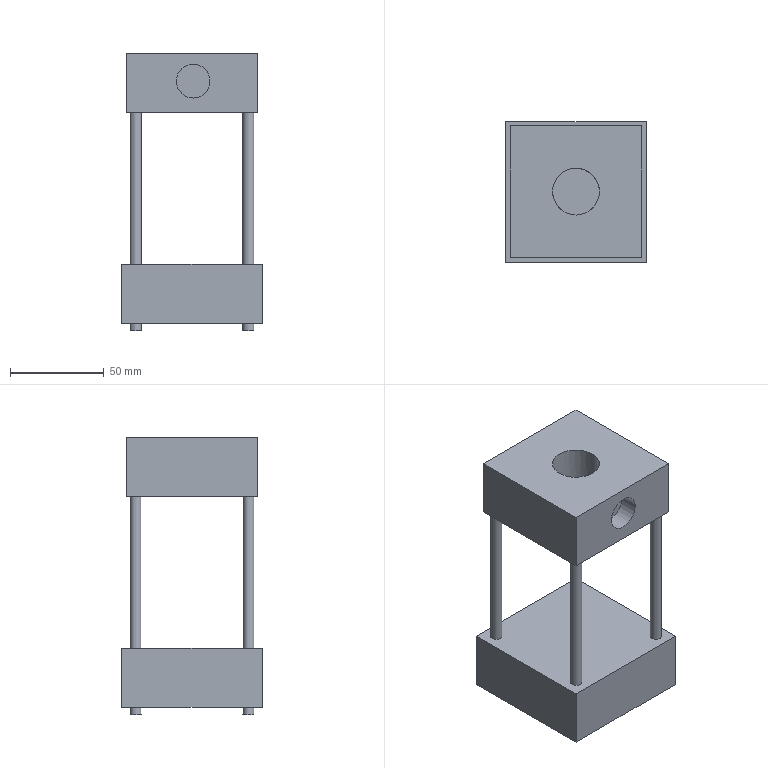Part | NX | features solid 2 | 1 solid | 27 faces | box 75 x 75 x 148 mm | volume 323144 mm3 | plane 17 | cylinder 10 | commonest cylinder face diameters 6 x8 18 x1 25 x1
STEP:
#1=CARTESIAN_POINT('',(33.,-470.,-344.));
#2=VERTEX_POINT('',#1);
#3=CARTESIAN_POINT('',(30.,-470.,-344.));
#4=DIRECTION('',(0.,0.,1.));
#5=DIRECTION('',(1.,0.,0.));
#6=AXIS2_PLACEMENT_3D('',#3,#4,#5);
#7=CIRCLE('',#6,3.);
#8=EDGE_CURVE('',#2,#2,#7,.T.);
#9=ORIENTED_EDGE('',*,*,#8,.T.);
#10=EDGE_LOOP('',(#9));
#11=FACE_BOUND('',#10,.T.);
#12=CARTESIAN_POINT('',(-27.,-410.,-344.));
#13=VERTEX_POINT('',#12);
#14=CARTESIAN_POINT('',(-30.,-410.,-344.));
#15=DIRECTION('',(0.,0.,1.));
#16=DIRECTION('',(1.,0.,0.));
#17=AXIS2_PLACEMENT_3D('',#14,#15,#16);
#18=CIRCLE('',#17,3.);
#19=EDGE_CURVE('',#13,#13,#18,.T.);
#20=ORIENTED_EDGE('',*,*,#19,.T.);
#21=EDGE_LOOP('',(#20));
#22=FACE_BOUND('',#21,.T.);
#23=CARTESIAN_POINT('',(-5.146,-477.5,-344.));
#24=VERTEX_POINT('',#23);
#25=CARTESIAN_POINT('',(-5.146,-465.,-344.));
#26=VERTEX_POINT('',#25);
#27=CARTESIAN_POINT('',(-5.146,-475.,-344.));
#28=DIRECTION('',(0.,1.,0.));
#29=VECTOR('',#28,1000.);
#30=LINE('',#27,#29);
#31=EDGE_CURVE('',#24,#26,#30,.T.);
#32=ORIENTED_EDGE('',*,*,#31,.F.);
#33=CARTESIAN_POINT('',(-37.5,-477.5,-344.));
#34=VERTEX_POINT('',#33);
#35=CARTESIAN_POINT('',(-35.,-477.5,-344.));
#36=DIRECTION('',(-1.,0.,0.));
#37=VECTOR('',#36,1000.);
#38=LINE('',#35,#37);
#39=EDGE_CURVE('',#24,#34,#38,.T.);
#40=ORIENTED_EDGE('',*,*,#39,.T.);
#41=CARTESIAN_POINT('',(-37.5,-402.5,-344.));
#42=VERTEX_POINT('',#41);
#43=CARTESIAN_POINT('',(-37.5,-475.,-344.));
#44=DIRECTION('',(0.,1.,0.));
#45=VECTOR('',#44,1000.);
#46=LINE('',#43,#45);
#47=EDGE_CURVE('',#42,#34,#46,.F.);
#48=ORIENTED_EDGE('',*,*,#47,.F.);
#49=CARTESIAN_POINT('',(37.5,-402.5,-344.));
#50=VERTEX_POINT('',#49);
#51=CARTESIAN_POINT('',(-35.,-402.5,-344.));
#52=DIRECTION('',(1.,0.,0.));
#53=VECTOR('',#52,1000.);
#54=LINE('',#51,#53);
#55=EDGE_CURVE('',#50,#42,#54,.F.);
#56=ORIENTED_EDGE('',*,*,#55,.F.);
#57=CARTESIAN_POINT('',(37.5,-477.5,-344.));
#58=VERTEX_POINT('',#57);
#59=CARTESIAN_POINT('',(37.5,-475.,-344.));
#60=DIRECTION('',(0.,-1.,0.));
#61=VECTOR('',#60,1000.);
#62=LINE('',#59,#61);
#63=EDGE_CURVE('',#58,#50,#62,.F.);
#64=ORIENTED_EDGE('',*,*,#63,.F.);
#65=CARTESIAN_POINT('',(3.1,-477.5,-344.));
#66=VERTEX_POINT('',#65);
#67=CARTESIAN_POINT('',(-35.,-477.5,-344.));
#68=DIRECTION('',(-1.,0.,0.));
#69=VECTOR('',#68,1000.);
#70=LINE('',#67,#69);
#71=EDGE_CURVE('',#58,#66,#70,.T.);
#72=ORIENTED_EDGE('',*,*,#71,.T.);
#73=CARTESIAN_POINT('',(3.1,-465.,-344.));
#74=VERTEX_POINT('',#73);
#75=CARTESIAN_POINT('',(3.1,-475.,-344.));
#76=DIRECTION('',(0.,1.,0.));
#77=VECTOR('',#76,1000.);
#78=LINE('',#75,#77);
#79=EDGE_CURVE('',#66,#74,#78,.T.);
#80=ORIENTED_EDGE('',*,*,#79,.T.);
#81=ORIENTED_EDGE('',*,*,#79,.F.);
#82=CARTESIAN_POINT('',(-35.,-477.5,-344.));
#83=DIRECTION('',(1.,0.,0.));
#84=VECTOR('',#83,1000.);
#85=LINE('',#82,#84);
#86=EDGE_CURVE('',#66,#24,#85,.F.);
#87=ORIENTED_EDGE('',*,*,#86,.T.);
#88=ORIENTED_EDGE('',*,*,#31,.T.);
#89=EDGE_LOOP('',(#32,#40,#48,#56,#64,#72,#80,#81,#87,#88));
#90=FACE_BOUND('',#89,.T.);
#91=CARTESIAN_POINT('',(-27.,-470.,-344.));
#92=VERTEX_POINT('',#91);
#93=CARTESIAN_POINT('',(-30.,-470.,-344.));
#94=DIRECTION('',(0.,0.,1.));
#95=DIRECTION('',(1.,0.,0.));
#96=AXIS2_PLACEMENT_3D('',#93,#94,#95);
#97=CIRCLE('',#96,3.);
#98=EDGE_CURVE('',#92,#92,#97,.T.);
#99=ORIENTED_EDGE('',*,*,#98,.T.);
#100=EDGE_LOOP('',(#99));
#101=FACE_BOUND('',#100,.T.);
#102=CARTESIAN_POINT('',(33.,-410.,-344.));
#103=VERTEX_POINT('',#102);
#104=CARTESIAN_POINT('',(30.,-410.,-344.));
#105=DIRECTION('',(0.,0.,1.));
#106=DIRECTION('',(1.,0.,0.));
#107=AXIS2_PLACEMENT_3D('',#104,#105,#106);
#108=CIRCLE('',#107,3.);
#109=EDGE_CURVE('',#103,#103,#108,.T.);
#110=ORIENTED_EDGE('',*,*,#109,.T.);
#111=EDGE_LOOP('',(#110));
#112=FACE_BOUND('',#111,.T.);
#113=CARTESIAN_POINT('',(-35.,-475.,-344.));
#114=DIRECTION('',(0.,0.,-1.));
#115=DIRECTION('',(1.,0.,0.));
#116=AXIS2_PLACEMENT_3D('',#113,#114,#115);
#117=PLANE('',#116);
#118=ADVANCED_FACE('',(#11,#22,#90,#101,#112),#117,.T.);
#119=CARTESIAN_POINT('',(-27.,-470.,-231.5));
#120=VERTEX_POINT('',#119);
#121=CARTESIAN_POINT('',(-30.,-470.,-231.5));
#122=DIRECTION('',(0.,0.,1.));
#123=DIRECTION('',(1.,0.,0.));
#124=AXIS2_PLACEMENT_3D('',#121,#122,#123);
#125=CIRCLE('',#124,3.);
#126=EDGE_CURVE('',#120,#120,#125,.T.);
#127=ORIENTED_EDGE('',*,*,#126,.F.);
#128=EDGE_LOOP('',(#127));
#129=FACE_BOUND('',#128,.T.);
#130=CARTESIAN_POINT('',(-27.,-470.,-312.5));
#131=VERTEX_POINT('',#130);
#132=CARTESIAN_POINT('',(-30.,-470.,-312.5));
#133=DIRECTION('',(0.,0.,1.));
#134=DIRECTION('',(1.,0.,0.));
#135=AXIS2_PLACEMENT_3D('',#132,#133,#134);
#136=CIRCLE('',#135,3.);
#137=EDGE_CURVE('',#131,#131,#136,.F.);
#138=ORIENTED_EDGE('',*,*,#137,.F.);
#139=EDGE_LOOP('',(#138));
#140=FACE_BOUND('',#139,.T.);
#141=CARTESIAN_POINT('',(-30.,-470.,-486.));
#142=DIRECTION('',(0.,0.,1.));
#143=DIRECTION('',(-1.,0.,0.));
#144=AXIS2_PLACEMENT_3D('',#141,#142,#143);
#145=CYLINDRICAL_SURFACE('',#144,3.);
#146=ADVANCED_FACE('',(#129,#140),#145,.T.);
#147=CARTESIAN_POINT('',(33.,-470.,-231.5));
#148=VERTEX_POINT('',#147);
#149=CARTESIAN_POINT('',(30.,-470.,-231.5));
#150=DIRECTION('',(0.,0.,1.));
#151=DIRECTION('',(1.,0.,0.));
#152=AXIS2_PLACEMENT_3D('',#149,#150,#151);
#153=CIRCLE('',#152,3.);
#154=EDGE_CURVE('',#148,#148,#153,.F.);
#155=ORIENTED_EDGE('',*,*,#154,.T.);
#156=EDGE_LOOP('',(#155));
#157=FACE_BOUND('',#156,.T.);
#158=CARTESIAN_POINT('',(33.,-470.,-312.5));
#159=VERTEX_POINT('',#158);
#160=CARTESIAN_POINT('',(30.,-470.,-312.5));
#161=DIRECTION('',(0.,0.,1.));
#162=DIRECTION('',(1.,0.,0.));
#163=AXIS2_PLACEMENT_3D('',#160,#161,#162);
#164=CIRCLE('',#163,3.);
#165=EDGE_CURVE('',#159,#159,#164,.T.);
#166=ORIENTED_EDGE('',*,*,#165,.T.);
#167=EDGE_LOOP('',(#166));
#168=FACE_BOUND('',#167,.T.);
#169=CARTESIAN_POINT('',(30.,-470.,-486.));
#170=DIRECTION('',(0.,0.,1.));
#171=DIRECTION('',(-1.,0.,0.));
#172=AXIS2_PLACEMENT_3D('',#169,#170,#171);
#173=CYLINDRICAL_SURFACE('',#172,3.);
#174=ADVANCED_FACE('',(#157,#168),#173,.T.);
#175=CARTESIAN_POINT('',(33.,-410.,-231.5));
#176=VERTEX_POINT('',#175);
#177=CARTESIAN_POINT('',(30.,-410.,-231.5));
#178=DIRECTION('',(0.,0.,1.));
#179=DIRECTION('',(1.,0.,0.));
#180=AXIS2_PLACEMENT_3D('',#177,#178,#179);
#181=CIRCLE('',#180,3.);
#182=EDGE_CURVE('',#176,#176,#181,.T.);
#183=ORIENTED_EDGE('',*,*,#182,.F.);
#184=EDGE_LOOP('',(#183));
#185=FACE_BOUND('',#184,.T.);
#186=CARTESIAN_POINT('',(33.,-410.,-312.5));
#187=VERTEX_POINT('',#186);
#188=CARTESIAN_POINT('',(30.,-410.,-312.5));
#189=DIRECTION('',(0.,0.,1.));
#190=DIRECTION('',(1.,0.,0.));
#191=AXIS2_PLACEMENT_3D('',#188,#189,#190);
#192=CIRCLE('',#191,3.);
#193=EDGE_CURVE('',#187,#187,#192,.F.);
#194=ORIENTED_EDGE('',*,*,#193,.F.);
#195=EDGE_LOOP('',(#194));
#196=FACE_BOUND('',#195,.T.);
#197=CARTESIAN_POINT('',(30.,-410.,-486.));
#198=DIRECTION('',(0.,0.,1.));
#199=DIRECTION('',(-1.,0.,0.));
#200=AXIS2_PLACEMENT_3D('',#197,#198,#199);
#201=CYLINDRICAL_SURFACE('',#200,3.);
#202=ADVANCED_FACE('',(#185,#196),#201,.T.);
#203=CARTESIAN_POINT('',(-27.,-410.,-231.5));
#204=VERTEX_POINT('',#203);
#205=CARTESIAN_POINT('',(-30.,-410.,-231.5));
#206=DIRECTION('',(0.,0.,1.));
#207=DIRECTION('',(1.,0.,0.));
#208=AXIS2_PLACEMENT_3D('',#205,#206,#207);
#209=CIRCLE('',#208,3.);
#210=EDGE_CURVE('',#204,#204,#209,.F.);
#211=ORIENTED_EDGE('',*,*,#210,.T.);
#212=EDGE_LOOP('',(#211));
#213=FACE_BOUND('',#212,.T.);
#214=CARTESIAN_POINT('',(-27.,-410.,-312.5));
#215=VERTEX_POINT('',#214);
#216=CARTESIAN_POINT('',(-30.,-410.,-312.5));
#217=DIRECTION('',(0.,0.,1.));
#218=DIRECTION('',(1.,0.,0.));
#219=AXIS2_PLACEMENT_3D('',#216,#217,#218);
#220=CIRCLE('',#219,3.);
#221=EDGE_CURVE('',#215,#215,#220,.T.);
#222=ORIENTED_EDGE('',*,*,#221,.T.);
#223=EDGE_LOOP('',(#222));
#224=FACE_BOUND('',#223,.T.);
#225=CARTESIAN_POINT('',(-30.,-410.,-486.));
#226=DIRECTION('',(0.,0.,1.));
#227=DIRECTION('',(-1.,0.,0.));
#228=AXIS2_PLACEMENT_3D('',#225,#226,#227);
#229=CYLINDRICAL_SURFACE('',#228,3.);
#230=ADVANCED_FACE('',(#213,#224),#229,.T.);
#231=ORIENTED_EDGE('',*,*,#154,.F.);
#232=EDGE_LOOP('',(#231));
#233=FACE_BOUND('',#232,.T.);
#234=ORIENTED_EDGE('',*,*,#126,.T.);
#235=EDGE_LOOP('',(#234));
#236=FACE_BOUND('',#235,.T.);
#237=CARTESIAN_POINT('',(12.5,-440.,-231.5));
#238=VERTEX_POINT('',#237);
#239=CARTESIAN_POINT('',(0.,-440.,-231.5));
#240=DIRECTION('',(0.,0.,1.));
#241=DIRECTION('',(1.,0.,0.));
#242=AXIS2_PLACEMENT_3D('',#239,#240,#241);
#243=CIRCLE('',#242,12.5);
#244=EDGE_CURVE('',#238,#238,#243,.T.);
#245=ORIENTED_EDGE('',*,*,#244,.T.);
#246=EDGE_LOOP('',(#245));
#247=FACE_BOUND('',#246,.T.);
#248=CARTESIAN_POINT('',(35.,-475.,-231.5));
#249=VERTEX_POINT('',#248);
#250=CARTESIAN_POINT('',(35.,-405.,-231.5));
#251=VERTEX_POINT('',#250);
#252=CARTESIAN_POINT('',(35.,-475.,-231.5));
#253=DIRECTION('',(0.,1.,0.));
#254=VECTOR('',#253,1000.);
#255=LINE('',#252,#254);
#256=EDGE_CURVE('',#249,#251,#255,.T.);
#257=ORIENTED_EDGE('',*,*,#256,.F.);
#258=CARTESIAN_POINT('',(-35.,-475.,-231.5));
#259=VERTEX_POINT('',#258);
#260=CARTESIAN_POINT('',(-35.,-475.,-231.5));
#261=DIRECTION('',(1.,0.,0.));
#262=VECTOR('',#261,1000.);
#263=LINE('',#260,#262);
#264=EDGE_CURVE('',#259,#249,#263,.T.);
#265=ORIENTED_EDGE('',*,*,#264,.F.);
#266=CARTESIAN_POINT('',(-35.,-405.,-231.5));
#267=VERTEX_POINT('',#266);
#268=CARTESIAN_POINT('',(-35.,-405.,-231.5));
#269=DIRECTION('',(0.,-1.,0.));
#270=VECTOR('',#269,1000.);
#271=LINE('',#268,#270);
#272=EDGE_CURVE('',#267,#259,#271,.T.);
#273=ORIENTED_EDGE('',*,*,#272,.F.);
#274=CARTESIAN_POINT('',(35.,-405.,-231.5));
#275=DIRECTION('',(-1.,0.,0.));
#276=VECTOR('',#275,1000.);
#277=LINE('',#274,#276);
#278=EDGE_CURVE('',#251,#267,#277,.T.);
#279=ORIENTED_EDGE('',*,*,#278,.F.);
#280=EDGE_LOOP('',(#257,#265,#273,#279));
#281=FACE_BOUND('',#280,.T.);
#282=ORIENTED_EDGE('',*,*,#182,.T.);
#283=EDGE_LOOP('',(#282));
#284=FACE_BOUND('',#283,.T.);
#285=ORIENTED_EDGE('',*,*,#210,.F.);
#286=EDGE_LOOP('',(#285));
#287=FACE_BOUND('',#286,.T.);
#288=CARTESIAN_POINT('',(35.,-405.,-231.5));
#289=DIRECTION('',(0.,0.,-1.));
#290=DIRECTION('',(1.,0.,0.));
#291=AXIS2_PLACEMENT_3D('',#288,#289,#290);
#292=PLANE('',#291);
#293=ADVANCED_FACE('',(#233,#236,#247,#281,#284,#287),#292,.T.);
#294=CARTESIAN_POINT('',(35.,-475.,-200.));
#295=VERTEX_POINT('',#294);
#296=CARTESIAN_POINT('',(35.,-405.,-200.));
#297=VERTEX_POINT('',#296);
#298=CARTESIAN_POINT('',(35.,-475.,-200.));
#299=DIRECTION('',(0.,1.,0.));
#300=VECTOR('',#299,1000.);
#301=LINE('',#298,#300);
#302=EDGE_CURVE('',#295,#297,#301,.T.);
#303=ORIENTED_EDGE('',*,*,#302,.F.);
#304=CARTESIAN_POINT('',(35.,-475.,-230.));
#305=DIRECTION('',(0.,0.,1.));
#306=VECTOR('',#305,1000.);
#307=LINE('',#304,#306);
#308=EDGE_CURVE('',#249,#295,#307,.T.);
#309=ORIENTED_EDGE('',*,*,#308,.F.);
#310=ORIENTED_EDGE('',*,*,#256,.T.);
#311=CARTESIAN_POINT('',(35.,-405.,-230.));
#312=DIRECTION('',(0.,0.,1.));
#313=VECTOR('',#312,1000.);
#314=LINE('',#311,#313);
#315=EDGE_CURVE('',#251,#297,#314,.T.);
#316=ORIENTED_EDGE('',*,*,#315,.T.);
#317=EDGE_LOOP('',(#303,#309,#310,#316));
#318=FACE_BOUND('',#317,.T.);
#319=CARTESIAN_POINT('',(35.,-475.,-230.));
#320=DIRECTION('',(-1.,0.,0.));
#321=DIRECTION('',(0.,-1.,0.));
#322=AXIS2_PLACEMENT_3D('',#319,#320,#321);
#323=PLANE('',#322);
#324=ADVANCED_FACE('',(#318),#323,.F.);
#325=CARTESIAN_POINT('',(-35.,-405.,-200.));
#326=VERTEX_POINT('',#325);
#327=CARTESIAN_POINT('',(35.,-405.,-200.));
#328=DIRECTION('',(-1.,0.,0.));
#329=VECTOR('',#328,1000.);
#330=LINE('',#327,#329);
#331=EDGE_CURVE('',#297,#326,#330,.T.);
#332=ORIENTED_EDGE('',*,*,#331,.F.);
#333=ORIENTED_EDGE('',*,*,#315,.F.);
#334=ORIENTED_EDGE('',*,*,#278,.T.);
#335=CARTESIAN_POINT('',(-35.,-405.,-230.));
#336=DIRECTION('',(0.,0.,1.));
#337=VECTOR('',#336,1000.);
#338=LINE('',#335,#337);
#339=EDGE_CURVE('',#267,#326,#338,.T.);
#340=ORIENTED_EDGE('',*,*,#339,.T.);
#341=EDGE_LOOP('',(#332,#333,#334,#340));
#342=FACE_BOUND('',#341,.T.);
#343=CARTESIAN_POINT('',(35.,-405.,-230.));
#344=DIRECTION('',(0.,-1.,0.));
#345=DIRECTION('',(1.,0.,0.));
#346=AXIS2_PLACEMENT_3D('',#343,#344,#345);
#347=PLANE('',#346);
#348=ADVANCED_FACE('',(#342),#347,.F.);
#349=CARTESIAN_POINT('',(-35.,-475.,-200.));
#350=VERTEX_POINT('',#349);
#351=CARTESIAN_POINT('',(-35.,-405.,-200.));
#352=DIRECTION('',(0.,-1.,0.));
#353=VECTOR('',#352,1000.);
#354=LINE('',#351,#353);
#355=EDGE_CURVE('',#326,#350,#354,.T.);
#356=ORIENTED_EDGE('',*,*,#355,.F.);
#357=ORIENTED_EDGE('',*,*,#339,.F.);
#358=ORIENTED_EDGE('',*,*,#272,.T.);
#359=CARTESIAN_POINT('',(-35.,-475.,-230.));
#360=DIRECTION('',(0.,0.,1.));
#361=VECTOR('',#360,1000.);
#362=LINE('',#359,#361);
#363=EDGE_CURVE('',#259,#350,#362,.T.);
#364=ORIENTED_EDGE('',*,*,#363,.T.);
#365=EDGE_LOOP('',(#356,#357,#358,#364));
#366=FACE_BOUND('',#365,.T.);
#367=CARTESIAN_POINT('',(-35.,-405.,-230.));
#368=DIRECTION('',(1.,0.,0.));
#369=DIRECTION('',(0.,0.,1.));
#370=AXIS2_PLACEMENT_3D('',#367,#368,#369);
#371=PLANE('',#370);
#372=ADVANCED_FACE('',(#366),#371,.F.);
#373=ORIENTED_EDGE('',*,*,#244,.F.);
#374=EDGE_LOOP('',(#373));
#375=FACE_BOUND('',#374,.T.);
#376=CARTESIAN_POINT('',(0.,-452.5,-200.));
#377=VERTEX_POINT('',#376);
#378=CARTESIAN_POINT('',(0.,-440.,-200.));
#379=DIRECTION('',(0.,0.,1.));
#380=DIRECTION('',(0.,-1.,0.));
#381=AXIS2_PLACEMENT_3D('',#378,#379,#380);
#382=CIRCLE('',#381,12.5);
#383=EDGE_CURVE('',#377,#377,#382,.T.);
#384=ORIENTED_EDGE('',*,*,#383,.T.);
#385=EDGE_LOOP('',(#384));
#386=FACE_BOUND('',#385,.T.);
#387=CARTESIAN_POINT('',(0.,-440.,-230.));
#388=DIRECTION('',(0.,0.,1.));
#389=DIRECTION('',(-1.,0.,0.));
#390=AXIS2_PLACEMENT_3D('',#387,#388,#389);
#391=CYLINDRICAL_SURFACE('',#390,12.5);
#392=ADVANCED_FACE('',(#375,#386),#391,.F.);
#393=CARTESIAN_POINT('',(0.609,-475.,-224.));
#394=VERTEX_POINT('',#393);
#395=CARTESIAN_POINT('',(0.609,-475.,-215.));
#396=DIRECTION('',(0.,-1.,0.));
#397=DIRECTION('',(0.,0.,-1.));
#398=AXIS2_PLACEMENT_3D('',#395,#396,#397);
#399=CIRCLE('',#398,9.);
#400=EDGE_CURVE('',#394,#394,#399,.T.);
#401=ORIENTED_EDGE('',*,*,#400,.F.);
#402=EDGE_LOOP('',(#401));
#403=FACE_BOUND('',#402,.T.);
#404=CARTESIAN_POINT('',(-35.,-475.,-200.));
#405=DIRECTION('',(1.,0.,0.));
#406=VECTOR('',#405,1000.);
#407=LINE('',#404,#406);
#408=EDGE_CURVE('',#350,#295,#407,.T.);
#409=ORIENTED_EDGE('',*,*,#408,.F.);
#410=ORIENTED_EDGE('',*,*,#363,.F.);
#411=ORIENTED_EDGE('',*,*,#264,.T.);
#412=ORIENTED_EDGE('',*,*,#308,.T.);
#413=EDGE_LOOP('',(#409,#410,#411,#412));
#414=FACE_BOUND('',#413,.T.);
#415=CARTESIAN_POINT('',(-35.,-475.,-230.));
#416=DIRECTION('',(0.,1.,0.));
#417=DIRECTION('',(0.,0.,-1.));
#418=AXIS2_PLACEMENT_3D('',#415,#416,#417);
#419=PLANE('',#418);
#420=ADVANCED_FACE('',(#403,#414),#419,.F.);
#421=ORIENTED_EDGE('',*,*,#383,.F.);
#422=EDGE_LOOP('',(#421));
#423=FACE_BOUND('',#422,.T.);
#424=ORIENTED_EDGE('',*,*,#302,.T.);
#425=ORIENTED_EDGE('',*,*,#331,.T.);
#426=ORIENTED_EDGE('',*,*,#355,.T.);
#427=ORIENTED_EDGE('',*,*,#408,.T.);
#428=EDGE_LOOP('',(#424,#425,#426,#427));
#429=FACE_BOUND('',#428,.T.);
#430=CARTESIAN_POINT('',(35.,-405.,-200.));
#431=DIRECTION('',(0.,0.,-1.));
#432=DIRECTION('',(1.,0.,0.));
#433=AXIS2_PLACEMENT_3D('',#430,#431,#432);
#434=PLANE('',#433);
#435=ADVANCED_FACE('',(#423,#429),#434,.F.);
#436=ORIENTED_EDGE('',*,*,#137,.T.);
#437=EDGE_LOOP('',(#436));
#438=FACE_BOUND('',#437,.T.);
#439=ORIENTED_EDGE('',*,*,#221,.F.);
#440=EDGE_LOOP('',(#439));
#441=FACE_BOUND('',#440,.T.);
#442=CARTESIAN_POINT('',(-37.5,-402.5,-312.5));
#443=VERTEX_POINT('',#442);
#444=CARTESIAN_POINT('',(-37.5,-477.5,-312.5));
#445=VERTEX_POINT('',#444);
#446=CARTESIAN_POINT('',(-37.5,-405.,-312.5));
#447=DIRECTION('',(0.,-1.,0.));
#448=VECTOR('',#447,1000.);
#449=LINE('',#446,#448);
#450=EDGE_CURVE('',#443,#445,#449,.T.);
#451=ORIENTED_EDGE('',*,*,#450,.T.);
#452=CARTESIAN_POINT('',(37.5,-477.5,-312.5));
#453=VERTEX_POINT('',#452);
#454=CARTESIAN_POINT('',(-35.,-477.5,-312.5));
#455=DIRECTION('',(1.,0.,0.));
#456=VECTOR('',#455,1000.);
#457=LINE('',#454,#456);
#458=EDGE_CURVE('',#445,#453,#457,.T.);
#459=ORIENTED_EDGE('',*,*,#458,.T.);
#460=CARTESIAN_POINT('',(37.5,-402.5,-312.5));
#461=VERTEX_POINT('',#460);
#462=CARTESIAN_POINT('',(37.5,-475.,-312.5));
#463=DIRECTION('',(0.,1.,0.));
#464=VECTOR('',#463,1000.);
#465=LINE('',#462,#464);
#466=EDGE_CURVE('',#453,#461,#465,.T.);
#467=ORIENTED_EDGE('',*,*,#466,.T.);
#468=CARTESIAN_POINT('',(35.,-402.5,-312.5));
#469=DIRECTION('',(-1.,0.,0.));
#470=VECTOR('',#469,1000.);
#471=LINE('',#468,#470);
#472=EDGE_CURVE('',#461,#443,#471,.T.);
#473=ORIENTED_EDGE('',*,*,#472,.T.);
#474=EDGE_LOOP('',(#451,#459,#467,#473));
#475=FACE_BOUND('',#474,.T.);
#476=ORIENTED_EDGE('',*,*,#193,.T.);
#477=EDGE_LOOP('',(#476));
#478=FACE_BOUND('',#477,.T.);
#479=ORIENTED_EDGE('',*,*,#165,.F.);
#480=EDGE_LOOP('',(#479));
#481=FACE_BOUND('',#480,.T.);
#482=CARTESIAN_POINT('',(-35.,-475.,-312.5));
#483=DIRECTION('',(0.,0.,-1.));
#484=DIRECTION('',(1.,0.,0.));
#485=AXIS2_PLACEMENT_3D('',#482,#483,#484);
#486=PLANE('',#485);
#487=ADVANCED_FACE('',(#438,#441,#475,#478,#481),#486,.F.);
#488=ORIENTED_EDGE('',*,*,#450,.F.);
#489=CARTESIAN_POINT('',(-37.5,-402.5,-481.));
#490=DIRECTION('',(0.,0.,1.));
#491=VECTOR('',#490,1000.);
#492=LINE('',#489,#491);
#493=EDGE_CURVE('',#42,#443,#492,.T.);
#494=ORIENTED_EDGE('',*,*,#493,.F.);
#495=ORIENTED_EDGE('',*,*,#47,.T.);
#496=CARTESIAN_POINT('',(-37.5,-477.5,-481.));
#497=DIRECTION('',(0.,0.,1.));
#498=VECTOR('',#497,1000.);
#499=LINE('',#496,#498);
#500=EDGE_CURVE('',#34,#445,#499,.T.);
#501=ORIENTED_EDGE('',*,*,#500,.T.);
#502=EDGE_LOOP('',(#488,#494,#495,#501));
#503=FACE_BOUND('',#502,.T.);
#504=CARTESIAN_POINT('',(-37.5,-405.,-481.));
#505=DIRECTION('',(1.,0.,0.));
#506=DIRECTION('',(0.,0.,1.));
#507=AXIS2_PLACEMENT_3D('',#504,#505,#506);
#508=PLANE('',#507);
#509=ADVANCED_FACE('',(#503),#508,.F.);
#510=ORIENTED_EDGE('',*,*,#458,.F.);
#511=ORIENTED_EDGE('',*,*,#500,.F.);
#512=ORIENTED_EDGE('',*,*,#39,.F.);
#513=ORIENTED_EDGE('',*,*,#86,.F.);
#514=ORIENTED_EDGE('',*,*,#71,.F.);
#515=CARTESIAN_POINT('',(37.5,-477.5,-481.));
#516=DIRECTION('',(0.,0.,1.));
#517=VECTOR('',#516,1000.);
#518=LINE('',#515,#517);
#519=EDGE_CURVE('',#58,#453,#518,.T.);
#520=ORIENTED_EDGE('',*,*,#519,.T.);
#521=EDGE_LOOP('',(#510,#511,#512,#513,#514,#520));
#522=FACE_BOUND('',#521,.T.);
#523=CARTESIAN_POINT('',(-35.,-477.5,-481.));
#524=DIRECTION('',(0.,1.,0.));
#525=DIRECTION('',(0.,0.,-1.));
#526=AXIS2_PLACEMENT_3D('',#523,#524,#525);
#527=PLANE('',#526);
#528=ADVANCED_FACE('',(#522),#527,.F.);
#529=ORIENTED_EDGE('',*,*,#466,.F.);
#530=ORIENTED_EDGE('',*,*,#519,.F.);
#531=ORIENTED_EDGE('',*,*,#63,.T.);
#532=CARTESIAN_POINT('',(37.5,-402.5,-481.));
#533=DIRECTION('',(0.,0.,1.));
#534=VECTOR('',#533,1000.);
#535=LINE('',#532,#534);
#536=EDGE_CURVE('',#50,#461,#535,.T.);
#537=ORIENTED_EDGE('',*,*,#536,.T.);
#538=EDGE_LOOP('',(#529,#530,#531,#537));
#539=FACE_BOUND('',#538,.T.);
#540=CARTESIAN_POINT('',(37.5,-475.,-481.));
#541=DIRECTION('',(-1.,0.,0.));
#542=DIRECTION('',(0.,-1.,0.));
#543=AXIS2_PLACEMENT_3D('',#540,#541,#542);
#544=PLANE('',#543);
#545=ADVANCED_FACE('',(#539),#544,.F.);
#546=ORIENTED_EDGE('',*,*,#472,.F.);
#547=ORIENTED_EDGE('',*,*,#536,.F.);
#548=ORIENTED_EDGE('',*,*,#55,.T.);
#549=ORIENTED_EDGE('',*,*,#493,.T.);
#550=EDGE_LOOP('',(#546,#547,#548,#549));
#551=FACE_BOUND('',#550,.T.);
#552=CARTESIAN_POINT('',(35.,-402.5,-481.));
#553=DIRECTION('',(0.,-1.,0.));
#554=DIRECTION('',(1.,0.,0.));
#555=AXIS2_PLACEMENT_3D('',#552,#553,#554);
#556=PLANE('',#555);
#557=ADVANCED_FACE('',(#551),#556,.F.);
#558=CARTESIAN_POINT('',(0.609,-465.,-224.));
#559=VERTEX_POINT('',#558);
#560=CARTESIAN_POINT('',(0.609,-465.,-215.));
#561=DIRECTION('',(0.,-1.,0.));
#562=DIRECTION('',(0.,0.,-1.));
#563=AXIS2_PLACEMENT_3D('',#560,#561,#562);
#564=CIRCLE('',#563,9.);
#565=EDGE_CURVE('',#559,#559,#564,.T.);
#566=ORIENTED_EDGE('',*,*,#565,.T.);
#567=EDGE_LOOP('',(#566));
#568=FACE_BOUND('',#567,.T.);
#569=CARTESIAN_POINT('',(0.609,-465.,-215.));
#570=DIRECTION('',(0.,1.,0.));
#571=DIRECTION('',(0.,0.,-1.));
#572=AXIS2_PLACEMENT_3D('',#569,#570,#571);
#573=PLANE('',#572);
#574=ADVANCED_FACE('',(#568),#573,.F.);
#575=ORIENTED_EDGE('',*,*,#565,.F.);
#576=EDGE_LOOP('',(#575));
#577=FACE_BOUND('',#576,.T.);
#578=ORIENTED_EDGE('',*,*,#400,.T.);
#579=EDGE_LOOP('',(#578));
#580=FACE_BOUND('',#579,.T.);
#581=CARTESIAN_POINT('',(0.609,-475.,-215.));
#582=DIRECTION('',(0.,1.,0.));
#583=DIRECTION('',(0.,0.,-1.));
#584=AXIS2_PLACEMENT_3D('',#581,#582,#583);
#585=CYLINDRICAL_SURFACE('',#584,9.);
#586=ADVANCED_FACE('',(#577,#580),#585,.F.);
#587=CARTESIAN_POINT('',(-27.,-410.,-348.));
#588=VERTEX_POINT('',#587);
#589=CARTESIAN_POINT('',(-30.,-410.,-348.));
#590=DIRECTION('',(0.,0.,1.));
#591=DIRECTION('',(1.,0.,0.));
#592=AXIS2_PLACEMENT_3D('',#589,#590,#591);
#593=CIRCLE('',#592,3.);
#594=EDGE_CURVE('',#588,#588,#593,.T.);
#595=ORIENTED_EDGE('',*,*,#594,.T.);
#596=EDGE_LOOP('',(#595));
#597=FACE_BOUND('',#596,.T.);
#598=ORIENTED_EDGE('',*,*,#19,.F.);
#599=EDGE_LOOP('',(#598));
#600=FACE_BOUND('',#599,.T.);
#601=CARTESIAN_POINT('',(-30.,-410.,-368.));
#602=DIRECTION('',(0.,0.,1.));
#603=DIRECTION('',(-1.,0.,0.));
#604=AXIS2_PLACEMENT_3D('',#601,#602,#603);
#605=CYLINDRICAL_SURFACE('',#604,3.);
#606=ADVANCED_FACE('',(#597,#600),#605,.T.);
#607=ORIENTED_EDGE('',*,*,#594,.F.);
#608=EDGE_LOOP('',(#607));
#609=FACE_BOUND('',#608,.T.);
#610=CARTESIAN_POINT('',(-95.,-415.,-348.));
#611=DIRECTION('',(0.,0.,-1.));
#612=DIRECTION('',(1.,0.,0.));
#613=AXIS2_PLACEMENT_3D('',#610,#611,#612);
#614=PLANE('',#613);
#615=ADVANCED_FACE('',(#609),#614,.T.);
#616=CARTESIAN_POINT('',(-27.,-470.,-348.));
#617=VERTEX_POINT('',#616);
#618=CARTESIAN_POINT('',(-30.,-470.,-348.));
#619=DIRECTION('',(0.,0.,1.));
#620=DIRECTION('',(1.,0.,0.));
#621=AXIS2_PLACEMENT_3D('',#618,#619,#620);
#622=CIRCLE('',#621,3.);
#623=EDGE_CURVE('',#617,#617,#622,.T.);
#624=ORIENTED_EDGE('',*,*,#623,.T.);
#625=EDGE_LOOP('',(#624));
#626=FACE_BOUND('',#625,.T.);
#627=ORIENTED_EDGE('',*,*,#98,.F.);
#628=EDGE_LOOP('',(#627));
#629=FACE_BOUND('',#628,.T.);
#630=CARTESIAN_POINT('',(-30.,-470.,-368.));
#631=DIRECTION('',(0.,0.,1.));
#632=DIRECTION('',(-1.,0.,0.));
#633=AXIS2_PLACEMENT_3D('',#630,#631,#632);
#634=CYLINDRICAL_SURFACE('',#633,3.);
#635=ADVANCED_FACE('',(#626,#629),#634,.T.);
#636=ORIENTED_EDGE('',*,*,#623,.F.);
#637=EDGE_LOOP('',(#636));
#638=FACE_BOUND('',#637,.T.);
#639=CARTESIAN_POINT('',(-95.,-475.,-348.));
#640=DIRECTION('',(0.,0.,-1.));
#641=DIRECTION('',(1.,0.,0.));
#642=AXIS2_PLACEMENT_3D('',#639,#640,#641);
#643=PLANE('',#642);
#644=ADVANCED_FACE('',(#638),#643,.T.);
#645=CARTESIAN_POINT('',(33.,-470.,-348.));
#646=VERTEX_POINT('',#645);
#647=CARTESIAN_POINT('',(30.,-470.,-348.));
#648=DIRECTION('',(0.,0.,1.));
#649=DIRECTION('',(1.,0.,0.));
#650=AXIS2_PLACEMENT_3D('',#647,#648,#649);
#651=CIRCLE('',#650,3.);
#652=EDGE_CURVE('',#646,#646,#651,.T.);
#653=ORIENTED_EDGE('',*,*,#652,.T.);
#654=EDGE_LOOP('',(#653));
#655=FACE_BOUND('',#654,.T.);
#656=ORIENTED_EDGE('',*,*,#8,.F.);
#657=EDGE_LOOP('',(#656));
#658=FACE_BOUND('',#657,.T.);
#659=CARTESIAN_POINT('',(30.,-470.,-368.));
#660=DIRECTION('',(0.,0.,1.));
#661=DIRECTION('',(-1.,0.,0.));
#662=AXIS2_PLACEMENT_3D('',#659,#660,#661);
#663=CYLINDRICAL_SURFACE('',#662,3.);
#664=ADVANCED_FACE('',(#655,#658),#663,.T.);
#665=ORIENTED_EDGE('',*,*,#652,.F.);
#666=EDGE_LOOP('',(#665));
#667=FACE_BOUND('',#666,.T.);
#668=CARTESIAN_POINT('',(-35.,-475.,-348.));
#669=DIRECTION('',(0.,0.,-1.));
#670=DIRECTION('',(1.,0.,0.));
#671=AXIS2_PLACEMENT_3D('',#668,#669,#670);
#672=PLANE('',#671);
#673=ADVANCED_FACE('',(#667),#672,.T.);
#674=CARTESIAN_POINT('',(33.,-410.,-348.));
#675=VERTEX_POINT('',#674);
#676=CARTESIAN_POINT('',(30.,-410.,-348.));
#677=DIRECTION('',(0.,0.,1.));
#678=DIRECTION('',(1.,0.,0.));
#679=AXIS2_PLACEMENT_3D('',#676,#677,#678);
#680=CIRCLE('',#679,3.);
#681=EDGE_CURVE('',#675,#675,#680,.T.);
#682=ORIENTED_EDGE('',*,*,#681,.T.);
#683=EDGE_LOOP('',(#682));
#684=FACE_BOUND('',#683,.T.);
#685=ORIENTED_EDGE('',*,*,#109,.F.);
#686=EDGE_LOOP('',(#685));
#687=FACE_BOUND('',#686,.T.);
#688=CARTESIAN_POINT('',(30.,-410.,-368.));
#689=DIRECTION('',(0.,0.,1.));
#690=DIRECTION('',(-1.,0.,0.));
#691=AXIS2_PLACEMENT_3D('',#688,#689,#690);
#692=CYLINDRICAL_SURFACE('',#691,3.);
#693=ADVANCED_FACE('',(#684,#687),#692,.T.);
#694=ORIENTED_EDGE('',*,*,#681,.F.);
#695=EDGE_LOOP('',(#694));
#696=FACE_BOUND('',#695,.T.);
#697=CARTESIAN_POINT('',(-35.,-415.,-348.));
#698=DIRECTION('',(0.,0.,-1.));
#699=DIRECTION('',(1.,0.,0.));
#700=AXIS2_PLACEMENT_3D('',#697,#698,#699);
#701=PLANE('',#700);
#702=ADVANCED_FACE('',(#696),#701,.T.);
#703=CLOSED_SHELL('',(#118,#146,#174,#202,#230,#293,#324,#348,#372,#392,#420,#435,#487,#509,#528,#545,#557,#574,#586,#606,#615,#635,#644,#664,#673,#693,#702));
#704=MANIFOLD_SOLID_BREP('',#703);
#705=(LENGTH_UNIT()NAMED_UNIT(*)SI_UNIT(.MILLI.,.METRE.));
#706=UNCERTAINTY_MEASURE_WITH_UNIT(LENGTH_MEASURE(0.00001),#705,'','');
#707=(NAMED_UNIT(*)PLANE_ANGLE_UNIT()SI_UNIT($,.RADIAN.));
#708=(NAMED_UNIT(*)SI_UNIT($,.STERADIAN.)SOLID_ANGLE_UNIT());
#709=(GEOMETRIC_REPRESENTATION_CONTEXT(3)GLOBAL_UNCERTAINTY_ASSIGNED_CONTEXT((#706))GLOBAL_UNIT_ASSIGNED_CONTEXT((#705,#707,#708))REPRESENTATION_CONTEXT('',''));
#710=ADVANCED_BREP_SHAPE_REPRESENTATION('',(#704),#709);